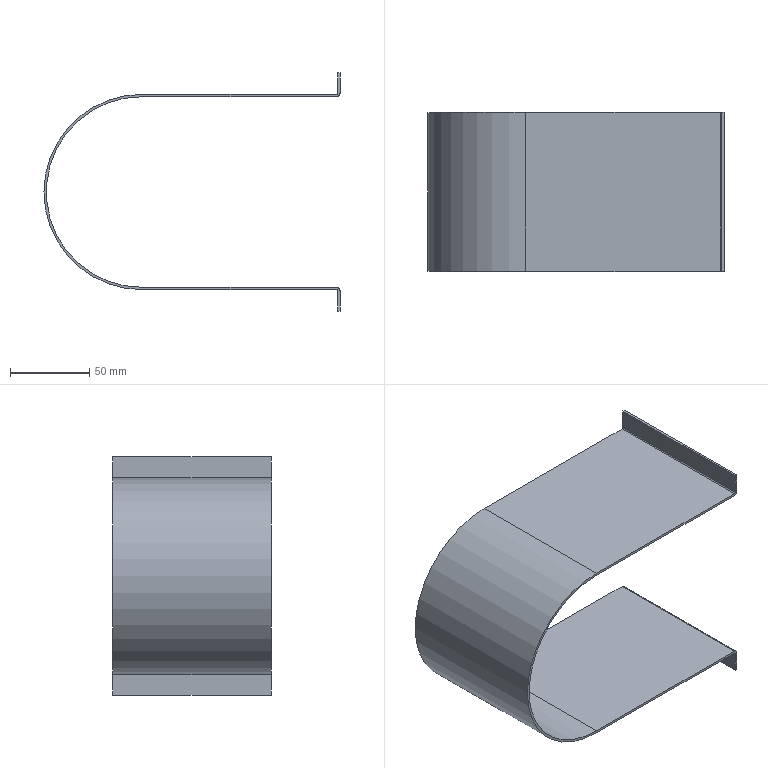Part | SolidWorks | features BaseBody 1 | 1 solid | 18 faces | box 186.5 x 100 x 150 mm | volume 69986 mm3 | plane 12 | cylinder 6 | commonest cylinder face diameters 1.473 x2 4.473 x2 120 x1 123 x1
STEP:
#1=CARTESIAN_POINT('',(-62.5,100.,61.5));
#2=VERTEX_POINT('',#1);
#3=CARTESIAN_POINT('',(-62.5,100.,-61.5));
#4=VERTEX_POINT('',#3);
#5=CARTESIAN_POINT('',(-62.5,100.,0.));
#6=DIRECTION('',(0.,-1.,0.));
#7=DIRECTION('',(0.,0.,-1.));
#8=AXIS2_PLACEMENT_3D('',#5,#6,#7);
#9=CIRCLE('',#8,61.5);
#10=EDGE_CURVE('',#2,#4,#9,.T.);
#11=ORIENTED_EDGE('',*,*,#10,.T.);
#12=CARTESIAN_POINT('',(-62.5,0.,-61.5));
#13=VERTEX_POINT('',#12);
#14=CARTESIAN_POINT('',(-62.5,100.,-61.5));
#15=DIRECTION('',(0.,-1.,0.));
#16=VECTOR('',#15,1000.);
#17=LINE('',#14,#16);
#18=EDGE_CURVE('',#4,#13,#17,.T.);
#19=ORIENTED_EDGE('',*,*,#18,.T.);
#20=CARTESIAN_POINT('',(-62.5,0.,61.5));
#21=VERTEX_POINT('',#20);
#22=CARTESIAN_POINT('',(-62.5,0.,0.));
#23=DIRECTION('',(0.,1.,0.));
#24=DIRECTION('',(0.,0.,-1.));
#25=AXIS2_PLACEMENT_3D('',#22,#23,#24);
#26=CIRCLE('',#25,61.5);
#27=EDGE_CURVE('',#13,#21,#26,.T.);
#28=ORIENTED_EDGE('',*,*,#27,.T.);
#29=CARTESIAN_POINT('',(-62.5,100.,61.5));
#30=DIRECTION('',(0.,1.,0.));
#31=VECTOR('',#30,1000.);
#32=LINE('',#29,#31);
#33=EDGE_CURVE('',#21,#2,#32,.T.);
#34=ORIENTED_EDGE('',*,*,#33,.T.);
#35=EDGE_LOOP('',(#11,#19,#28,#34));
#36=FACE_OUTER_BOUND('',#35,.T.);
#37=CARTESIAN_POINT('',(-62.5,100.,0.));
#38=DIRECTION('',(0.,-1.,0.));
#39=DIRECTION('',(0.,0.,-1.));
#40=AXIS2_PLACEMENT_3D('',#37,#38,#39);
#41=CYLINDRICAL_SURFACE('',#40,61.5);
#42=ADVANCED_FACE('',(#36),#41,.T.);
#43=ORIENTED_EDGE('',*,*,#18,.F.);
#44=CARTESIAN_POINT('',(60.263,100.,-61.5));
#45=VERTEX_POINT('',#44);
#46=CARTESIAN_POINT('',(-62.5,100.,-61.5));
#47=DIRECTION('',(-1.,0.,0.));
#48=VECTOR('',#47,1000.);
#49=LINE('',#46,#48);
#50=EDGE_CURVE('',#45,#4,#49,.T.);
#51=ORIENTED_EDGE('',*,*,#50,.F.);
#52=CARTESIAN_POINT('',(60.263,0.,-61.5));
#53=VERTEX_POINT('',#52);
#54=CARTESIAN_POINT('',(60.263,100.,-61.5));
#55=DIRECTION('',(0.,1.,0.));
#56=VECTOR('',#55,1000.);
#57=LINE('',#54,#56);
#58=EDGE_CURVE('',#53,#45,#57,.T.);
#59=ORIENTED_EDGE('',*,*,#58,.F.);
#60=CARTESIAN_POINT('',(-62.5,0.,-61.5));
#61=DIRECTION('',(1.,0.,0.));
#62=VECTOR('',#61,1000.);
#63=LINE('',#60,#62);
#64=EDGE_CURVE('',#13,#53,#63,.T.);
#65=ORIENTED_EDGE('',*,*,#64,.F.);
#66=EDGE_LOOP('',(#43,#51,#59,#65));
#67=FACE_OUTER_BOUND('',#66,.T.);
#68=CARTESIAN_POINT('',(-62.5,100.,-61.5));
#69=DIRECTION('',(0.,0.,1.));
#70=DIRECTION('',(1.,0.,0.));
#71=AXIS2_PLACEMENT_3D('',#68,#69,#70);
#72=PLANE('',#71);
#73=ADVANCED_FACE('',(#67),#72,.F.);
#74=CARTESIAN_POINT('',(-62.5,100.,60.));
#75=VERTEX_POINT('',#74);
#76=CARTESIAN_POINT('',(-62.5,100.,-60.));
#77=VERTEX_POINT('',#76);
#78=CARTESIAN_POINT('',(-62.5,100.,0.));
#79=DIRECTION('',(0.,-1.,0.));
#80=DIRECTION('',(0.,0.,-1.));
#81=AXIS2_PLACEMENT_3D('',#78,#79,#80);
#82=CIRCLE('',#81,60.);
#83=EDGE_CURVE('',#75,#77,#82,.T.);
#84=ORIENTED_EDGE('',*,*,#83,.T.);
#85=CARTESIAN_POINT('',(60.263,100.,-60.));
#86=VERTEX_POINT('',#85);
#87=CARTESIAN_POINT('',(61.,100.,-60.));
#88=DIRECTION('',(1.,0.,0.));
#89=VECTOR('',#88,1000.);
#90=LINE('',#87,#89);
#91=EDGE_CURVE('',#77,#86,#90,.T.);
#92=ORIENTED_EDGE('',*,*,#91,.T.);
#93=CARTESIAN_POINT('',(62.5,100.,-62.237));
#94=VERTEX_POINT('',#93);
#95=CARTESIAN_POINT('',(60.263,100.,-62.237));
#96=DIRECTION('',(0.,-1.,0.));
#97=DIRECTION('',(0.,0.,-1.));
#98=AXIS2_PLACEMENT_3D('',#95,#96,#97);
#99=CIRCLE('',#98,2.237);
#100=EDGE_CURVE('',#94,#86,#99,.T.);
#101=ORIENTED_EDGE('',*,*,#100,.F.);
#102=CARTESIAN_POINT('',(62.5,100.,-75.));
#103=VERTEX_POINT('',#102);
#104=CARTESIAN_POINT('',(62.5,100.,62.237));
#105=DIRECTION('',(0.,0.,-1.));
#106=VECTOR('',#105,1000.);
#107=LINE('',#104,#106);
#108=EDGE_CURVE('',#94,#103,#107,.T.);
#109=ORIENTED_EDGE('',*,*,#108,.T.);
#110=CARTESIAN_POINT('',(61.,100.,-75.));
#111=VERTEX_POINT('',#110);
#112=CARTESIAN_POINT('',(60.263,100.,-75.));
#113=DIRECTION('',(-1.,0.,0.));
#114=VECTOR('',#113,1000.);
#115=LINE('',#112,#114);
#116=EDGE_CURVE('',#103,#111,#115,.T.);
#117=ORIENTED_EDGE('',*,*,#116,.T.);
#118=CARTESIAN_POINT('',(61.,100.,-62.237));
#119=VERTEX_POINT('',#118);
#120=CARTESIAN_POINT('',(61.,100.,-60.));
#121=DIRECTION('',(0.,0.,1.));
#122=VECTOR('',#121,1000.);
#123=LINE('',#120,#122);
#124=EDGE_CURVE('',#111,#119,#123,.T.);
#125=ORIENTED_EDGE('',*,*,#124,.T.);
#126=CARTESIAN_POINT('',(60.263,100.,-62.237));
#127=DIRECTION('',(0.,-1.,0.));
#128=DIRECTION('',(0.,0.,-1.));
#129=AXIS2_PLACEMENT_3D('',#126,#127,#128);
#130=CIRCLE('',#129,0.7366);
#131=EDGE_CURVE('',#119,#45,#130,.T.);
#132=ORIENTED_EDGE('',*,*,#131,.T.);
#133=ORIENTED_EDGE('',*,*,#50,.T.);
#134=ORIENTED_EDGE('',*,*,#10,.F.);
#135=CARTESIAN_POINT('',(60.263,100.,61.5));
#136=VERTEX_POINT('',#135);
#137=CARTESIAN_POINT('',(-62.5,100.,61.5));
#138=DIRECTION('',(1.,0.,0.));
#139=VECTOR('',#138,1000.);
#140=LINE('',#137,#139);
#141=EDGE_CURVE('',#2,#136,#140,.T.);
#142=ORIENTED_EDGE('',*,*,#141,.T.);
#143=CARTESIAN_POINT('',(61.,100.,62.237));
#144=VERTEX_POINT('',#143);
#145=CARTESIAN_POINT('',(60.263,100.,62.237));
#146=DIRECTION('',(0.,-1.,0.));
#147=DIRECTION('',(0.,0.,-1.));
#148=AXIS2_PLACEMENT_3D('',#145,#146,#147);
#149=CIRCLE('',#148,0.7366);
#150=EDGE_CURVE('',#136,#144,#149,.T.);
#151=ORIENTED_EDGE('',*,*,#150,.T.);
#152=CARTESIAN_POINT('',(61.,100.,75.));
#153=VERTEX_POINT('',#152);
#154=CARTESIAN_POINT('',(61.,100.,60.));
#155=DIRECTION('',(0.,0.,1.));
#156=VECTOR('',#155,1000.);
#157=LINE('',#154,#156);
#158=EDGE_CURVE('',#144,#153,#157,.T.);
#159=ORIENTED_EDGE('',*,*,#158,.T.);
#160=CARTESIAN_POINT('',(62.5,100.,75.));
#161=VERTEX_POINT('',#160);
#162=CARTESIAN_POINT('',(62.5,100.,75.));
#163=DIRECTION('',(-1.,0.,0.));
#164=VECTOR('',#163,1000.);
#165=LINE('',#162,#164);
#166=EDGE_CURVE('',#161,#153,#165,.T.);
#167=ORIENTED_EDGE('',*,*,#166,.F.);
#168=CARTESIAN_POINT('',(62.5,100.,62.237));
#169=VERTEX_POINT('',#168);
#170=CARTESIAN_POINT('',(62.5,100.,61.5));
#171=DIRECTION('',(0.,0.,-1.));
#172=VECTOR('',#171,1000.);
#173=LINE('',#170,#172);
#174=EDGE_CURVE('',#161,#169,#173,.T.);
#175=ORIENTED_EDGE('',*,*,#174,.T.);
#176=CARTESIAN_POINT('',(60.263,100.,60.));
#177=VERTEX_POINT('',#176);
#178=CARTESIAN_POINT('',(60.263,100.,62.237));
#179=DIRECTION('',(0.,-1.,0.));
#180=DIRECTION('',(0.,0.,-1.));
#181=AXIS2_PLACEMENT_3D('',#178,#179,#180);
#182=CIRCLE('',#181,2.237);
#183=EDGE_CURVE('',#177,#169,#182,.T.);
#184=ORIENTED_EDGE('',*,*,#183,.F.);
#185=CARTESIAN_POINT('',(-62.5,100.,60.));
#186=DIRECTION('',(-1.,0.,0.));
#187=VECTOR('',#186,1000.);
#188=LINE('',#185,#187);
#189=EDGE_CURVE('',#177,#75,#188,.T.);
#190=ORIENTED_EDGE('',*,*,#189,.T.);
#191=EDGE_LOOP('',(#84,#92,#101,#109,#117,#125,#132,#133,#134,#142,#151,#159,#167,#175,#184,#190));
#192=FACE_OUTER_BOUND('',#191,.T.);
#193=CARTESIAN_POINT('',(-62.5,100.,60.));
#194=DIRECTION('',(0.,1.,0.));
#195=DIRECTION('',(0.,0.,1.));
#196=AXIS2_PLACEMENT_3D('',#193,#194,#195);
#197=PLANE('',#196);
#198=ADVANCED_FACE('',(#192),#197,.T.);
#199=CARTESIAN_POINT('',(60.263,0.,61.5));
#200=VERTEX_POINT('',#199);
#201=CARTESIAN_POINT('',(60.263,100.,61.5));
#202=DIRECTION('',(0.,-1.,0.));
#203=VECTOR('',#202,1000.);
#204=LINE('',#201,#203);
#205=EDGE_CURVE('',#136,#200,#204,.T.);
#206=ORIENTED_EDGE('',*,*,#205,.F.);
#207=ORIENTED_EDGE('',*,*,#141,.F.);
#208=ORIENTED_EDGE('',*,*,#33,.F.);
#209=CARTESIAN_POINT('',(-62.5,0.,61.5));
#210=DIRECTION('',(-1.,0.,0.));
#211=VECTOR('',#210,1000.);
#212=LINE('',#209,#211);
#213=EDGE_CURVE('',#200,#21,#212,.T.);
#214=ORIENTED_EDGE('',*,*,#213,.F.);
#215=EDGE_LOOP('',(#206,#207,#208,#214));
#216=FACE_OUTER_BOUND('',#215,.T.);
#217=CARTESIAN_POINT('',(-62.5,100.,61.5));
#218=DIRECTION('',(0.,0.,-1.));
#219=DIRECTION('',(-1.,0.,0.));
#220=AXIS2_PLACEMENT_3D('',#217,#218,#219);
#221=PLANE('',#220);
#222=ADVANCED_FACE('',(#216),#221,.F.);
#223=CARTESIAN_POINT('',(-62.5,0.,-60.));
#224=VERTEX_POINT('',#223);
#225=CARTESIAN_POINT('',(-62.5,0.,60.));
#226=VERTEX_POINT('',#225);
#227=CARTESIAN_POINT('',(-62.5,0.,0.));
#228=DIRECTION('',(0.,1.,0.));
#229=DIRECTION('',(0.,0.,-1.));
#230=AXIS2_PLACEMENT_3D('',#227,#228,#229);
#231=CIRCLE('',#230,60.);
#232=EDGE_CURVE('',#224,#226,#231,.T.);
#233=ORIENTED_EDGE('',*,*,#232,.T.);
#234=CARTESIAN_POINT('',(60.263,0.,60.));
#235=VERTEX_POINT('',#234);
#236=CARTESIAN_POINT('',(61.,0.,60.));
#237=DIRECTION('',(1.,0.,0.));
#238=VECTOR('',#237,1000.);
#239=LINE('',#236,#238);
#240=EDGE_CURVE('',#226,#235,#239,.T.);
#241=ORIENTED_EDGE('',*,*,#240,.T.);
#242=CARTESIAN_POINT('',(62.5,0.,62.237));
#243=VERTEX_POINT('',#242);
#244=CARTESIAN_POINT('',(60.263,0.,62.237));
#245=DIRECTION('',(0.,1.,0.));
#246=DIRECTION('',(0.,0.,-1.));
#247=AXIS2_PLACEMENT_3D('',#244,#245,#246);
#248=CIRCLE('',#247,2.237);
#249=EDGE_CURVE('',#243,#235,#248,.T.);
#250=ORIENTED_EDGE('',*,*,#249,.F.);
#251=CARTESIAN_POINT('',(62.5,0.,75.));
#252=VERTEX_POINT('',#251);
#253=CARTESIAN_POINT('',(62.5,0.,62.237));
#254=DIRECTION('',(0.,0.,-1.));
#255=VECTOR('',#254,1000.);
#256=LINE('',#253,#255);
#257=EDGE_CURVE('',#252,#243,#256,.T.);
#258=ORIENTED_EDGE('',*,*,#257,.F.);
#259=CARTESIAN_POINT('',(61.,0.,75.));
#260=VERTEX_POINT('',#259);
#261=CARTESIAN_POINT('',(60.263,0.,75.));
#262=DIRECTION('',(1.,0.,0.));
#263=VECTOR('',#262,1000.);
#264=LINE('',#261,#263);
#265=EDGE_CURVE('',#260,#252,#264,.T.);
#266=ORIENTED_EDGE('',*,*,#265,.F.);
#267=CARTESIAN_POINT('',(61.,0.,62.237));
#268=VERTEX_POINT('',#267);
#269=CARTESIAN_POINT('',(61.,0.,60.));
#270=DIRECTION('',(0.,0.,-1.));
#271=VECTOR('',#270,1000.);
#272=LINE('',#269,#271);
#273=EDGE_CURVE('',#260,#268,#272,.T.);
#274=ORIENTED_EDGE('',*,*,#273,.T.);
#275=CARTESIAN_POINT('',(60.263,0.,62.237));
#276=DIRECTION('',(0.,1.,0.));
#277=DIRECTION('',(0.,0.,-1.));
#278=AXIS2_PLACEMENT_3D('',#275,#276,#277);
#279=CIRCLE('',#278,0.7366);
#280=EDGE_CURVE('',#268,#200,#279,.T.);
#281=ORIENTED_EDGE('',*,*,#280,.T.);
#282=ORIENTED_EDGE('',*,*,#213,.T.);
#283=ORIENTED_EDGE('',*,*,#27,.F.);
#284=ORIENTED_EDGE('',*,*,#64,.T.);
#285=CARTESIAN_POINT('',(61.,0.,-62.237));
#286=VERTEX_POINT('',#285);
#287=CARTESIAN_POINT('',(60.263,0.,-62.237));
#288=DIRECTION('',(0.,1.,0.));
#289=DIRECTION('',(0.,0.,-1.));
#290=AXIS2_PLACEMENT_3D('',#287,#288,#289);
#291=CIRCLE('',#290,0.7366);
#292=EDGE_CURVE('',#53,#286,#291,.T.);
#293=ORIENTED_EDGE('',*,*,#292,.T.);
#294=CARTESIAN_POINT('',(61.,0.,-75.));
#295=VERTEX_POINT('',#294);
#296=CARTESIAN_POINT('',(61.,0.,-60.));
#297=DIRECTION('',(0.,0.,-1.));
#298=VECTOR('',#297,1000.);
#299=LINE('',#296,#298);
#300=EDGE_CURVE('',#286,#295,#299,.T.);
#301=ORIENTED_EDGE('',*,*,#300,.T.);
#302=CARTESIAN_POINT('',(62.5,0.,-75.));
#303=VERTEX_POINT('',#302);
#304=CARTESIAN_POINT('',(60.263,0.,-75.));
#305=DIRECTION('',(1.,0.,0.));
#306=VECTOR('',#305,1000.);
#307=LINE('',#304,#306);
#308=EDGE_CURVE('',#295,#303,#307,.T.);
#309=ORIENTED_EDGE('',*,*,#308,.T.);
#310=CARTESIAN_POINT('',(62.5,0.,-62.237));
#311=VERTEX_POINT('',#310);
#312=CARTESIAN_POINT('',(62.5,0.,-61.5));
#313=DIRECTION('',(0.,0.,1.));
#314=VECTOR('',#313,1000.);
#315=LINE('',#312,#314);
#316=EDGE_CURVE('',#303,#311,#315,.T.);
#317=ORIENTED_EDGE('',*,*,#316,.T.);
#318=CARTESIAN_POINT('',(60.263,0.,-60.));
#319=VERTEX_POINT('',#318);
#320=CARTESIAN_POINT('',(60.263,0.,-62.237));
#321=DIRECTION('',(0.,1.,0.));
#322=DIRECTION('',(0.,0.,-1.));
#323=AXIS2_PLACEMENT_3D('',#320,#321,#322);
#324=CIRCLE('',#323,2.237);
#325=EDGE_CURVE('',#319,#311,#324,.T.);
#326=ORIENTED_EDGE('',*,*,#325,.F.);
#327=CARTESIAN_POINT('',(-62.5,0.,-60.));
#328=DIRECTION('',(-1.,0.,0.));
#329=VECTOR('',#328,1000.);
#330=LINE('',#327,#329);
#331=EDGE_CURVE('',#319,#224,#330,.T.);
#332=ORIENTED_EDGE('',*,*,#331,.T.);
#333=EDGE_LOOP('',(#233,#241,#250,#258,#266,#274,#281,#282,#283,#284,#293,#301,#309,#317,#326,#332));
#334=FACE_OUTER_BOUND('',#333,.T.);
#335=CARTESIAN_POINT('',(-62.5,0.,-60.));
#336=DIRECTION('',(0.,-1.,0.));
#337=DIRECTION('',(0.,0.,-1.));
#338=AXIS2_PLACEMENT_3D('',#335,#336,#337);
#339=PLANE('',#338);
#340=ADVANCED_FACE('',(#334),#339,.T.);
#341=ORIENTED_EDGE('',*,*,#58,.T.);
#342=ORIENTED_EDGE('',*,*,#131,.F.);
#343=CARTESIAN_POINT('',(61.,100.,-62.237));
#344=DIRECTION('',(0.,1.,0.));
#345=VECTOR('',#344,1000.);
#346=LINE('',#343,#345);
#347=EDGE_CURVE('',#286,#119,#346,.T.);
#348=ORIENTED_EDGE('',*,*,#347,.F.);
#349=ORIENTED_EDGE('',*,*,#292,.F.);
#350=EDGE_LOOP('',(#341,#342,#348,#349));
#351=FACE_OUTER_BOUND('',#350,.T.);
#352=CARTESIAN_POINT('',(60.263,100.,-62.237));
#353=DIRECTION('',(0.,-1.,0.));
#354=DIRECTION('',(0.,0.,-1.));
#355=AXIS2_PLACEMENT_3D('',#352,#353,#354);
#356=CYLINDRICAL_SURFACE('',#355,0.7366);
#357=ADVANCED_FACE('',(#351),#356,.F.);
#358=CARTESIAN_POINT('',(-62.5,100.,-60.));
#359=DIRECTION('',(0.,-1.,0.));
#360=VECTOR('',#359,1000.);
#361=LINE('',#358,#360);
#362=EDGE_CURVE('',#77,#224,#361,.T.);
#363=ORIENTED_EDGE('',*,*,#362,.F.);
#364=ORIENTED_EDGE('',*,*,#83,.F.);
#365=CARTESIAN_POINT('',(-62.5,100.,60.));
#366=DIRECTION('',(0.,1.,0.));
#367=VECTOR('',#366,1000.);
#368=LINE('',#365,#367);
#369=EDGE_CURVE('',#226,#75,#368,.T.);
#370=ORIENTED_EDGE('',*,*,#369,.F.);
#371=ORIENTED_EDGE('',*,*,#232,.F.);
#372=EDGE_LOOP('',(#363,#364,#370,#371));
#373=FACE_OUTER_BOUND('',#372,.T.);
#374=CARTESIAN_POINT('',(-62.5,100.,0.));
#375=DIRECTION('',(0.,-1.,0.));
#376=DIRECTION('',(0.,0.,-1.));
#377=AXIS2_PLACEMENT_3D('',#374,#375,#376);
#378=CYLINDRICAL_SURFACE('',#377,60.);
#379=ADVANCED_FACE('',(#373),#378,.F.);
#380=CARTESIAN_POINT('',(61.,100.,62.237));
#381=DIRECTION('',(0.,-1.,0.));
#382=VECTOR('',#381,1000.);
#383=LINE('',#380,#382);
#384=EDGE_CURVE('',#144,#268,#383,.T.);
#385=ORIENTED_EDGE('',*,*,#384,.F.);
#386=ORIENTED_EDGE('',*,*,#150,.F.);
#387=ORIENTED_EDGE('',*,*,#205,.T.);
#388=ORIENTED_EDGE('',*,*,#280,.F.);
#389=EDGE_LOOP('',(#385,#386,#387,#388));
#390=FACE_OUTER_BOUND('',#389,.T.);
#391=CARTESIAN_POINT('',(60.263,100.,62.237));
#392=DIRECTION('',(0.,-1.,0.));
#393=DIRECTION('',(0.,0.,-1.));
#394=AXIS2_PLACEMENT_3D('',#391,#392,#393);
#395=CYLINDRICAL_SURFACE('',#394,0.7366);
#396=ADVANCED_FACE('',(#390),#395,.F.);
#397=ORIENTED_EDGE('',*,*,#91,.F.);
#398=ORIENTED_EDGE('',*,*,#362,.T.);
#399=ORIENTED_EDGE('',*,*,#331,.F.);
#400=CARTESIAN_POINT('',(60.263,100.,-60.));
#401=DIRECTION('',(0.,1.,0.));
#402=VECTOR('',#401,1000.);
#403=LINE('',#400,#402);
#404=EDGE_CURVE('',#319,#86,#403,.T.);
#405=ORIENTED_EDGE('',*,*,#404,.T.);
#406=EDGE_LOOP('',(#397,#398,#399,#405));
#407=FACE_OUTER_BOUND('',#406,.T.);
#408=CARTESIAN_POINT('',(-62.5,100.,-60.));
#409=DIRECTION('',(0.,0.,1.));
#410=DIRECTION('',(1.,0.,0.));
#411=AXIS2_PLACEMENT_3D('',#408,#409,#410);
#412=PLANE('',#411);
#413=ADVANCED_FACE('',(#407),#412,.T.);
#414=ORIENTED_EDGE('',*,*,#347,.T.);
#415=ORIENTED_EDGE('',*,*,#124,.F.);
#416=CARTESIAN_POINT('',(61.,100.,-75.));
#417=DIRECTION('',(0.,1.,0.));
#418=VECTOR('',#417,1000.);
#419=LINE('',#416,#418);
#420=EDGE_CURVE('',#295,#111,#419,.T.);
#421=ORIENTED_EDGE('',*,*,#420,.F.);
#422=ORIENTED_EDGE('',*,*,#300,.F.);
#423=EDGE_LOOP('',(#414,#415,#421,#422));
#424=FACE_OUTER_BOUND('',#423,.T.);
#425=CARTESIAN_POINT('',(61.,100.,-60.));
#426=DIRECTION('',(1.,0.,0.));
#427=DIRECTION('',(0.,0.,-1.));
#428=AXIS2_PLACEMENT_3D('',#425,#426,#427);
#429=PLANE('',#428);
#430=ADVANCED_FACE('',(#424),#429,.F.);
#431=ORIENTED_EDGE('',*,*,#189,.F.);
#432=CARTESIAN_POINT('',(60.263,100.,60.));
#433=DIRECTION('',(0.,-1.,0.));
#434=VECTOR('',#433,1000.);
#435=LINE('',#432,#434);
#436=EDGE_CURVE('',#177,#235,#435,.T.);
#437=ORIENTED_EDGE('',*,*,#436,.T.);
#438=ORIENTED_EDGE('',*,*,#240,.F.);
#439=ORIENTED_EDGE('',*,*,#369,.T.);
#440=EDGE_LOOP('',(#431,#437,#438,#439));
#441=FACE_OUTER_BOUND('',#440,.T.);
#442=CARTESIAN_POINT('',(-62.5,100.,60.));
#443=DIRECTION('',(0.,0.,-1.));
#444=DIRECTION('',(-1.,0.,0.));
#445=AXIS2_PLACEMENT_3D('',#442,#443,#444);
#446=PLANE('',#445);
#447=ADVANCED_FACE('',(#441),#446,.T.);
#448=CARTESIAN_POINT('',(61.,100.,75.));
#449=DIRECTION('',(0.,-1.,0.));
#450=VECTOR('',#449,1000.);
#451=LINE('',#448,#450);
#452=EDGE_CURVE('',#153,#260,#451,.T.);
#453=ORIENTED_EDGE('',*,*,#452,.F.);
#454=ORIENTED_EDGE('',*,*,#158,.F.);
#455=ORIENTED_EDGE('',*,*,#384,.T.);
#456=ORIENTED_EDGE('',*,*,#273,.F.);
#457=EDGE_LOOP('',(#453,#454,#455,#456));
#458=FACE_OUTER_BOUND('',#457,.T.);
#459=CARTESIAN_POINT('',(61.,100.,60.));
#460=DIRECTION('',(1.,0.,0.));
#461=DIRECTION('',(0.,0.,-1.));
#462=AXIS2_PLACEMENT_3D('',#459,#460,#461);
#463=PLANE('',#462);
#464=ADVANCED_FACE('',(#458),#463,.F.);
#465=ORIENTED_EDGE('',*,*,#100,.T.);
#466=ORIENTED_EDGE('',*,*,#404,.F.);
#467=ORIENTED_EDGE('',*,*,#325,.T.);
#468=CARTESIAN_POINT('',(62.5,100.,-62.237));
#469=DIRECTION('',(0.,1.,0.));
#470=VECTOR('',#469,1000.);
#471=LINE('',#468,#470);
#472=EDGE_CURVE('',#311,#94,#471,.T.);
#473=ORIENTED_EDGE('',*,*,#472,.T.);
#474=EDGE_LOOP('',(#465,#466,#467,#473));
#475=FACE_OUTER_BOUND('',#474,.T.);
#476=CARTESIAN_POINT('',(60.263,100.,-62.237));
#477=DIRECTION('',(0.,-1.,0.));
#478=DIRECTION('',(0.,0.,-1.));
#479=AXIS2_PLACEMENT_3D('',#476,#477,#478);
#480=CYLINDRICAL_SURFACE('',#479,2.237);
#481=ADVANCED_FACE('',(#475),#480,.T.);
#482=ORIENTED_EDGE('',*,*,#116,.F.);
#483=CARTESIAN_POINT('',(62.5,100.,-75.));
#484=DIRECTION('',(0.,-1.,0.));
#485=VECTOR('',#484,1000.);
#486=LINE('',#483,#485);
#487=EDGE_CURVE('',#103,#303,#486,.T.);
#488=ORIENTED_EDGE('',*,*,#487,.T.);
#489=ORIENTED_EDGE('',*,*,#308,.F.);
#490=ORIENTED_EDGE('',*,*,#420,.T.);
#491=EDGE_LOOP('',(#482,#488,#489,#490));
#492=FACE_OUTER_BOUND('',#491,.T.);
#493=CARTESIAN_POINT('',(61.,100.,-75.));
#494=DIRECTION('',(0.,0.,-1.));
#495=DIRECTION('',(-1.,0.,0.));
#496=AXIS2_PLACEMENT_3D('',#493,#494,#495);
#497=PLANE('',#496);
#498=ADVANCED_FACE('',(#492),#497,.T.);
#499=ORIENTED_EDGE('',*,*,#183,.T.);
#500=CARTESIAN_POINT('',(62.5,100.,62.237));
#501=DIRECTION('',(0.,-1.,0.));
#502=VECTOR('',#501,1000.);
#503=LINE('',#500,#502);
#504=EDGE_CURVE('',#169,#243,#503,.T.);
#505=ORIENTED_EDGE('',*,*,#504,.T.);
#506=ORIENTED_EDGE('',*,*,#249,.T.);
#507=ORIENTED_EDGE('',*,*,#436,.F.);
#508=EDGE_LOOP('',(#499,#505,#506,#507));
#509=FACE_OUTER_BOUND('',#508,.T.);
#510=CARTESIAN_POINT('',(60.263,100.,62.237));
#511=DIRECTION('',(0.,-1.,0.));
#512=DIRECTION('',(0.,0.,-1.));
#513=AXIS2_PLACEMENT_3D('',#510,#511,#512);
#514=CYLINDRICAL_SURFACE('',#513,2.237);
#515=ADVANCED_FACE('',(#509),#514,.T.);
#516=ORIENTED_EDGE('',*,*,#166,.T.);
#517=ORIENTED_EDGE('',*,*,#452,.T.);
#518=ORIENTED_EDGE('',*,*,#265,.T.);
#519=CARTESIAN_POINT('',(62.5,100.,75.));
#520=DIRECTION('',(0.,1.,0.));
#521=VECTOR('',#520,1000.);
#522=LINE('',#519,#521);
#523=EDGE_CURVE('',#252,#161,#522,.T.);
#524=ORIENTED_EDGE('',*,*,#523,.T.);
#525=EDGE_LOOP('',(#516,#517,#518,#524));
#526=FACE_OUTER_BOUND('',#525,.T.);
#527=CARTESIAN_POINT('',(62.5,100.,75.));
#528=DIRECTION('',(0.,0.,1.));
#529=DIRECTION('',(1.,0.,0.));
#530=AXIS2_PLACEMENT_3D('',#527,#528,#529);
#531=PLANE('',#530);
#532=ADVANCED_FACE('',(#526),#531,.T.);
#533=ORIENTED_EDGE('',*,*,#108,.F.);
#534=ORIENTED_EDGE('',*,*,#472,.F.);
#535=ORIENTED_EDGE('',*,*,#316,.F.);
#536=ORIENTED_EDGE('',*,*,#487,.F.);
#537=EDGE_LOOP('',(#533,#534,#535,#536));
#538=FACE_OUTER_BOUND('',#537,.T.);
#539=CARTESIAN_POINT('',(62.5,100.,-60.));
#540=DIRECTION('',(1.,0.,0.));
#541=DIRECTION('',(0.,0.,-1.));
#542=AXIS2_PLACEMENT_3D('',#539,#540,#541);
#543=PLANE('',#542);
#544=ADVANCED_FACE('',(#538),#543,.T.);
#545=ORIENTED_EDGE('',*,*,#174,.F.);
#546=ORIENTED_EDGE('',*,*,#523,.F.);
#547=ORIENTED_EDGE('',*,*,#257,.T.);
#548=ORIENTED_EDGE('',*,*,#504,.F.);
#549=EDGE_LOOP('',(#545,#546,#547,#548));
#550=FACE_OUTER_BOUND('',#549,.T.);
#551=CARTESIAN_POINT('',(62.5,100.,60.));
#552=DIRECTION('',(1.,0.,0.));
#553=DIRECTION('',(0.,0.,-1.));
#554=AXIS2_PLACEMENT_3D('',#551,#552,#553);
#555=PLANE('',#554);
#556=ADVANCED_FACE('',(#550),#555,.T.);
#557=CLOSED_SHELL('',(#42,#73,#198,#222,#340,#357,#379,#396,#413,#430,#447,#464,#481,#498,#515,#532,#544,#556));
#558=MANIFOLD_SOLID_BREP('',#557);
#559=CARTESIAN_POINT('',(0.,0.,0.));
#560=DIRECTION('',(0.,0.,1.));
#561=DIRECTION('',(1.,0.,0.));
#562=AXIS2_PLACEMENT_3D('',#559,#560,#561);
#563=(LENGTH_UNIT()NAMED_UNIT(*)SI_UNIT(.MILLI.,.METRE.));
#564=UNCERTAINTY_MEASURE_WITH_UNIT(LENGTH_MEASURE(0.00001),#563,'','');
#565=(NAMED_UNIT(*)PLANE_ANGLE_UNIT()SI_UNIT($,.RADIAN.));
#566=(NAMED_UNIT(*)SI_UNIT($,.STERADIAN.)SOLID_ANGLE_UNIT());
#567=(GEOMETRIC_REPRESENTATION_CONTEXT(3)GLOBAL_UNCERTAINTY_ASSIGNED_CONTEXT((#564))GLOBAL_UNIT_ASSIGNED_CONTEXT((#563,#565,#566))REPRESENTATION_CONTEXT('',''));
#568=ADVANCED_BREP_SHAPE_REPRESENTATION('',(#558,#562),#567);